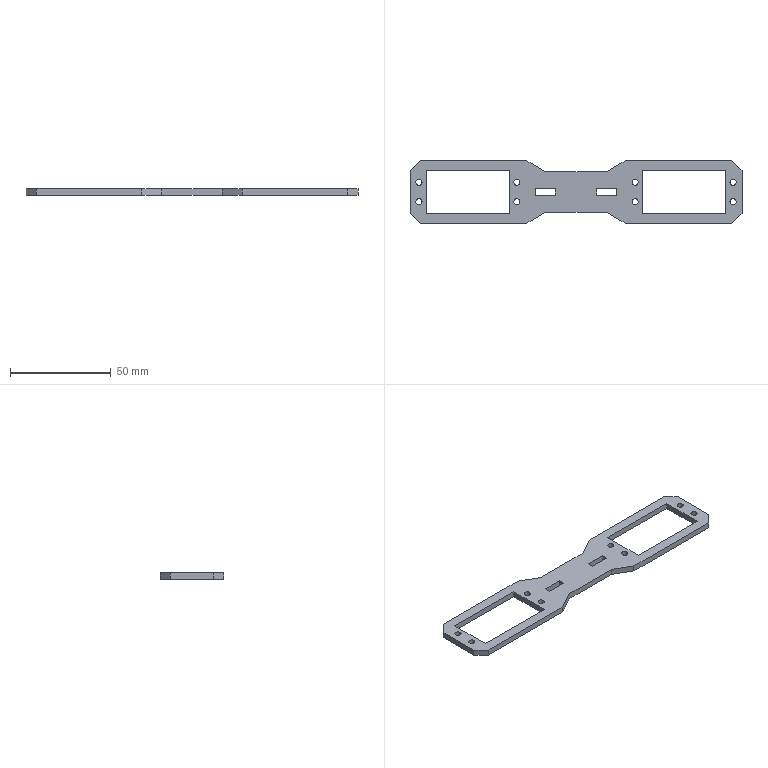Part | SolidWorks | features Extrusion 1 | 1 solid | 50 faces | box 164.86 x 31.5 x 3 mm | volume 8343 mm3 | plane 34 | cylinder 16 | commonest cylinder face diameters 3.05 x16